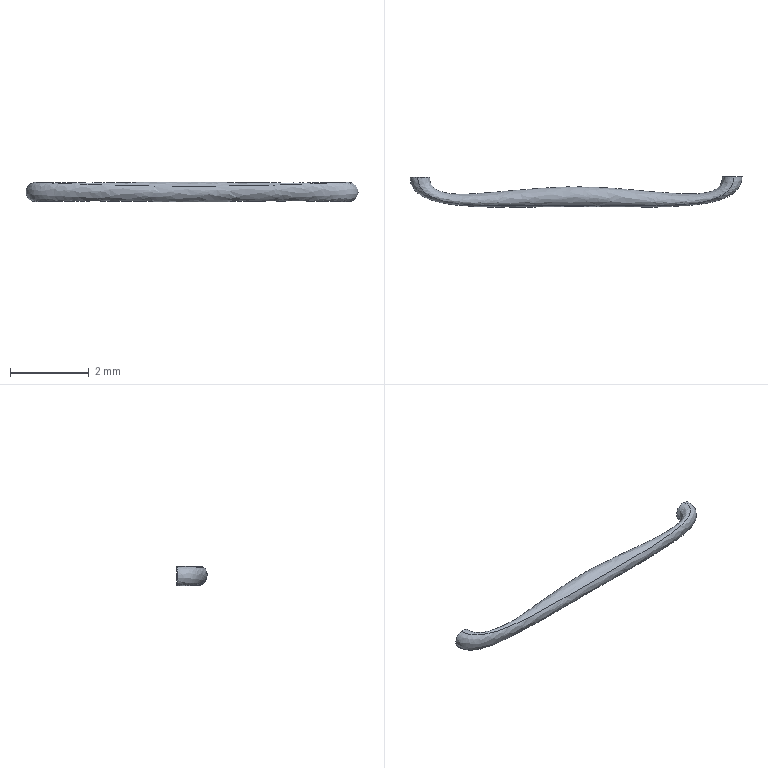Part | SolidWorks | features BaseBody 1 | 1 solid | 4 faces | box 8.423 x 0.7721 x 0.5 mm | volume 1.254 mm3 | plane 2 | spline 2
STEP:
#1=CARTESIAN_POINT('',(345.954,392.468,98.256));
#2=VERTEX_POINT('',#1);
#3=CARTESIAN_POINT('',(345.875,392.468,97.762));
#4=VERTEX_POINT('',#3);
#5=CARTESIAN_POINT('',(345.954,392.468,98.256));
#6=CARTESIAN_POINT('',(345.961,392.468,98.255));
#7=CARTESIAN_POINT('',(345.975,392.468,98.252));
#8=CARTESIAN_POINT('',(345.994,392.468,98.246));
#9=CARTESIAN_POINT('',(346.013,392.468,98.239));
#10=CARTESIAN_POINT('',(346.072,392.468,98.211));
#11=CARTESIAN_POINT('',(346.132,392.468,98.149));
#12=CARTESIAN_POINT('',(346.165,392.468,98.05));
#13=CARTESIAN_POINT('',(346.166,392.468,97.961));
#14=CARTESIAN_POINT('',(346.132,392.468,97.872));
#15=CARTESIAN_POINT('',(346.064,392.468,97.801));
#16=CARTESIAN_POINT('',(345.976,392.468,97.76));
#17=CARTESIAN_POINT('',(345.908,392.468,97.757));
#18=CARTESIAN_POINT('',(345.875,392.468,97.762));
#19=B_SPLINE_CURVE_WITH_KNOTS('',3,(#5,#6,#7,#8,#9,#10,#11,#12,#13,#14,#15,#16,#17,#18),.UNSPECIFIED.,.F.,.F.,(4,1,1,1,1,1,1,1,1,1,1,4),(0.,0.025,0.05,0.075,0.1,0.3,0.4,0.5,0.625,0.75,0.875,1.),.UNSPECIFIED.);
#20=EDGE_CURVE('',#2,#4,#19,.T.);
#21=ORIENTED_EDGE('',*,*,#20,.T.);
#22=CARTESIAN_POINT('',(345.875,392.468,97.762));
#23=CARTESIAN_POINT('',(345.842,392.468,97.767));
#24=CARTESIAN_POINT('',(345.778,392.468,97.792));
#25=CARTESIAN_POINT('',(345.707,392.468,97.859));
#26=CARTESIAN_POINT('',(345.666,392.468,97.947));
#27=CARTESIAN_POINT('',(345.661,392.468,98.043));
#28=CARTESIAN_POINT('',(345.69,392.468,98.127));
#29=CARTESIAN_POINT('',(345.752,392.468,98.21));
#30=CARTESIAN_POINT('',(345.829,392.468,98.25));
#31=CARTESIAN_POINT('',(345.894,392.468,98.258));
#32=CARTESIAN_POINT('',(345.914,392.468,98.259));
#33=CARTESIAN_POINT('',(345.934,392.468,98.258));
#34=CARTESIAN_POINT('',(345.948,392.468,98.257));
#35=CARTESIAN_POINT('',(345.954,392.468,98.256));
#36=B_SPLINE_CURVE_WITH_KNOTS('',3,(#22,#23,#24,#25,#26,#27,#28,#29,#30,#31,#32,#33,#34,#35),.UNSPECIFIED.,.F.,.F.,(4,1,1,1,1,1,1,1,1,1,1,4),(0.,0.125,0.25,0.375,0.5,0.6,0.7,0.9,0.925,0.95,0.975,1.),.UNSPECIFIED.);
#37=EDGE_CURVE('',#4,#2,#36,.T.);
#38=ORIENTED_EDGE('',*,*,#37,.T.);
#39=EDGE_LOOP('',(#21,#38));
#40=FACE_OUTER_BOUND('',#39,.T.);
#41=CARTESIAN_POINT('',(345.915,392.468,98.009));
#42=DIRECTION('',(0.0009599,-1.,0.));
#43=DIRECTION('',(0.,0.,-1.));
#44=AXIS2_PLACEMENT_3D('',#41,#42,#43);
#45=PLANE('',#44);
#46=ADVANCED_FACE('',(#40),#45,.F.);
#47=CARTESIAN_POINT('',(337.94,392.46,98.253));
#48=VERTEX_POINT('',#47);
#49=CARTESIAN_POINT('',(338.044,392.46,97.764));
#50=VERTEX_POINT('',#49);
#51=CARTESIAN_POINT('',(337.94,392.46,98.253));
#52=CARTESIAN_POINT('',(337.946,392.46,98.255));
#53=CARTESIAN_POINT('',(337.96,392.46,98.257));
#54=CARTESIAN_POINT('',(337.98,392.46,98.259));
#55=CARTESIAN_POINT('',(338.,392.46,98.259));
#56=CARTESIAN_POINT('',(338.065,392.46,98.254));
#57=CARTESIAN_POINT('',(338.144,392.46,98.218));
#58=CARTESIAN_POINT('',(338.211,392.46,98.138));
#59=CARTESIAN_POINT('',(338.243,392.46,98.056));
#60=CARTESIAN_POINT('',(338.244,392.46,97.96));
#61=CARTESIAN_POINT('',(338.207,392.46,97.87));
#62=CARTESIAN_POINT('',(338.14,392.46,97.799));
#63=CARTESIAN_POINT('',(338.077,392.46,97.771));
#64=CARTESIAN_POINT('',(338.044,392.46,97.764));
#65=B_SPLINE_CURVE_WITH_KNOTS('',3,(#51,#52,#53,#54,#55,#56,#57,#58,#59,#60,#61,#62,#63,#64),.UNSPECIFIED.,.F.,.F.,(4,1,1,1,1,1,1,1,1,1,1,4),(0.,0.025,0.05,0.075,0.1,0.3,0.4,0.5,0.625,0.75,0.875,1.),.UNSPECIFIED.);
#66=EDGE_CURVE('',#48,#50,#65,.T.);
#67=ORIENTED_EDGE('',*,*,#66,.T.);
#68=CARTESIAN_POINT('',(338.044,392.46,97.764));
#69=CARTESIAN_POINT('',(338.011,392.46,97.757));
#70=CARTESIAN_POINT('',(337.943,392.46,97.757));
#71=CARTESIAN_POINT('',(337.853,392.46,97.794));
#72=CARTESIAN_POINT('',(337.782,392.46,97.861));
#73=CARTESIAN_POINT('',(337.743,392.46,97.949));
#74=CARTESIAN_POINT('',(337.739,392.46,98.038));
#75=CARTESIAN_POINT('',(337.767,392.46,98.138));
#76=CARTESIAN_POINT('',(337.824,392.46,98.203));
#77=CARTESIAN_POINT('',(337.882,392.46,98.234));
#78=CARTESIAN_POINT('',(337.901,392.46,98.242));
#79=CARTESIAN_POINT('',(337.92,392.46,98.248));
#80=CARTESIAN_POINT('',(337.933,392.46,98.252));
#81=CARTESIAN_POINT('',(337.94,392.46,98.253));
#82=B_SPLINE_CURVE_WITH_KNOTS('',3,(#68,#69,#70,#71,#72,#73,#74,#75,#76,#77,#78,#79,#80,#81),.UNSPECIFIED.,.F.,.F.,(4,1,1,1,1,1,1,1,1,1,1,4),(0.,0.125,0.25,0.375,0.5,0.6,0.7,0.9,0.925,0.95,0.975,1.),.UNSPECIFIED.);
#83=EDGE_CURVE('',#50,#48,#82,.T.);
#84=ORIENTED_EDGE('',*,*,#83,.T.);
#85=EDGE_LOOP('',(#67,#84));
#86=FACE_OUTER_BOUND('',#85,.T.);
#87=CARTESIAN_POINT('',(337.992,392.46,98.009));
#88=DIRECTION('',(0.0009599,-1.,0.));
#89=DIRECTION('',(0.,0.,-1.));
#90=AXIS2_PLACEMENT_3D('',#87,#88,#89);
#91=PLANE('',#90);
#92=ADVANCED_FACE('',(#86),#91,.F.);
#93=CARTESIAN_POINT('',(338.044,392.46,97.764));
#94=CARTESIAN_POINT('',(338.045,391.637,97.764));
#95=CARTESIAN_POINT('',(341.947,392.702,97.981));
#96=CARTESIAN_POINT('',(345.876,391.642,97.762));
#97=CARTESIAN_POINT('',(345.875,392.468,97.762));
#98=B_SPLINE_CURVE_WITH_KNOTS('',3,(#93,#94,#95,#96,#97),.UNSPECIFIED.,.F.,.F.,(4,1,4),(0.,0.5,1.),.UNSPECIFIED.);
#99=EDGE_CURVE('',#50,#4,#98,.T.);
#100=ORIENTED_EDGE('',*,*,#99,.T.);
#101=ORIENTED_EDGE('',*,*,#20,.F.);
#102=CARTESIAN_POINT('',(345.954,392.468,98.256));
#103=CARTESIAN_POINT('',(345.955,391.561,98.256));
#104=CARTESIAN_POINT('',(341.96,391.959,98.052));
#105=CARTESIAN_POINT('',(337.94,391.551,98.253));
#106=CARTESIAN_POINT('',(337.94,392.46,98.253));
#107=B_SPLINE_CURVE_WITH_KNOTS('',3,(#102,#103,#104,#105,#106),.UNSPECIFIED.,.F.,.F.,(4,1,4),(0.,0.5,1.),.UNSPECIFIED.);
#108=EDGE_CURVE('',#2,#48,#107,.T.);
#109=ORIENTED_EDGE('',*,*,#108,.T.);
#110=ORIENTED_EDGE('',*,*,#83,.F.);
#111=EDGE_LOOP('',(#100,#101,#109,#110));
#112=FACE_OUTER_BOUND('',#111,.T.);
#113=CARTESIAN_POINT('',(337.961,392.546,98.256));
#114=CARTESIAN_POINT('',(337.834,391.542,98.262));
#115=CARTESIAN_POINT('',(341.966,391.986,98.069));
#116=CARTESIAN_POINT('',(346.071,391.552,98.264));
#117=CARTESIAN_POINT('',(345.932,392.561,98.257));
#118=CARTESIAN_POINT('',(337.955,392.546,98.255));
#119=CARTESIAN_POINT('',(337.828,391.541,98.261));
#120=CARTESIAN_POINT('',(341.966,391.981,98.061));
#121=CARTESIAN_POINT('',(346.077,391.55,98.264));
#122=CARTESIAN_POINT('',(345.937,392.561,98.257));
#123=CARTESIAN_POINT('',(337.944,392.547,98.253));
#124=CARTESIAN_POINT('',(337.816,391.538,98.259));
#125=CARTESIAN_POINT('',(341.966,391.97,98.043));
#126=CARTESIAN_POINT('',(346.089,391.547,98.263));
#127=CARTESIAN_POINT('',(345.949,392.562,98.255));
#128=CARTESIAN_POINT('',(337.925,392.547,98.248));
#129=CARTESIAN_POINT('',(337.797,391.532,98.255));
#130=CARTESIAN_POINT('',(341.965,391.955,98.014));
#131=CARTESIAN_POINT('',(346.108,391.542,98.26));
#132=CARTESIAN_POINT('',(345.968,392.562,98.251));
#133=CARTESIAN_POINT('',(337.906,392.548,98.242));
#134=CARTESIAN_POINT('',(337.777,391.527,98.25));
#135=CARTESIAN_POINT('',(341.965,391.942,97.984));
#136=CARTESIAN_POINT('',(346.128,391.537,98.255));
#137=CARTESIAN_POINT('',(345.987,392.563,98.246));
#138=CARTESIAN_POINT('',(337.888,392.548,98.233));
#139=CARTESIAN_POINT('',(337.759,391.522,98.242));
#140=CARTESIAN_POINT('',(341.965,391.932,97.954));
#141=CARTESIAN_POINT('',(346.148,391.532,98.248));
#142=CARTESIAN_POINT('',(346.006,392.563,98.239));
#143=CARTESIAN_POINT('',(337.83,392.55,98.202));
#144=CARTESIAN_POINT('',(337.699,391.508,98.213));
#145=CARTESIAN_POINT('',(341.964,391.906,97.856));
#146=CARTESIAN_POINT('',(346.209,391.517,98.223));
#147=CARTESIAN_POINT('',(346.065,392.565,98.21));
#148=CARTESIAN_POINT('',(337.773,392.55,98.137));
#149=CARTESIAN_POINT('',(337.64,391.497,98.149));
#150=CARTESIAN_POINT('',(341.963,391.924,97.745));
#151=CARTESIAN_POINT('',(346.271,391.505,98.162));
#152=CARTESIAN_POINT('',(346.125,392.566,98.148));
#153=CARTESIAN_POINT('',(337.745,392.55,98.037));
#154=CARTESIAN_POINT('',(337.611,391.497,98.049));
#155=CARTESIAN_POINT('',(341.96,392.023,97.662));
#156=CARTESIAN_POINT('',(346.306,391.504,98.063));
#157=CARTESIAN_POINT('',(346.158,392.566,98.05));
#158=CARTESIAN_POINT('',(337.749,392.549,97.948));
#159=CARTESIAN_POINT('',(337.616,391.504,97.958));
#160=CARTESIAN_POINT('',(341.958,392.145,97.629));
#161=CARTESIAN_POINT('',(346.306,391.51,97.972));
#162=CARTESIAN_POINT('',(346.159,392.565,97.961));
#163=CARTESIAN_POINT('',(337.788,392.548,97.861));
#164=CARTESIAN_POINT('',(337.656,391.522,97.867));
#165=CARTESIAN_POINT('',(341.955,392.305,97.648));
#166=CARTESIAN_POINT('',(346.271,391.527,97.879));
#167=CARTESIAN_POINT('',(346.125,392.563,97.872));
#168=CARTESIAN_POINT('',(337.858,392.545,97.794));
#169=CARTESIAN_POINT('',(337.729,391.548,97.796));
#170=CARTESIAN_POINT('',(341.953,392.474,97.722));
#171=CARTESIAN_POINT('',(346.201,391.552,97.804));
#172=CARTESIAN_POINT('',(346.058,392.56,97.801));
#173=CARTESIAN_POINT('',(337.948,392.542,97.757));
#174=CARTESIAN_POINT('',(337.821,391.578,97.755));
#175=CARTESIAN_POINT('',(341.952,392.626,97.837));
#176=CARTESIAN_POINT('',(346.111,391.58,97.757));
#177=CARTESIAN_POINT('',(345.97,392.557,97.76));
#178=CARTESIAN_POINT('',(338.022,392.54,97.758));
#179=CARTESIAN_POINT('',(337.897,391.597,97.752));
#180=CARTESIAN_POINT('',(341.951,392.713,97.945));
#181=CARTESIAN_POINT('',(346.034,391.6,97.75));
#182=CARTESIAN_POINT('',(345.896,392.555,97.757));
#183=CARTESIAN_POINT('',(338.06,392.539,97.767));
#184=CARTESIAN_POINT('',(337.936,391.606,97.76));
#185=CARTESIAN_POINT('',(341.951,392.745,98.003));
#186=CARTESIAN_POINT('',(345.995,391.609,97.756));
#187=CARTESIAN_POINT('',(345.858,392.554,97.764));
#188=CARTESIAN_POINT('',(338.064,392.539,97.768));
#189=CARTESIAN_POINT('',(337.941,391.607,97.761));
#190=CARTESIAN_POINT('',(341.951,392.749,98.011));
#191=CARTESIAN_POINT('',(345.99,391.61,97.757));
#192=CARTESIAN_POINT('',(345.853,392.554,97.765));
#193=B_SPLINE_SURFACE_WITH_KNOTS('',3,3,((#113,#114,#115,#116,#117),(#118,#119,#120,#121,#122),(#123,#124,#125,#126,#127),(#128,#129,#130,#131,#132),(#133,#134,#135,#136,#137),(#138,#139,#140,#141,#142),(#143,#144,#145,#146,#147),(#148,#149,#150,#151,#152),(#153,#154,#155,#156,#157),(#158,#159,#160,#161,#162),(#163,#164,#165,#166,#167),(#168,#169,#170,#171,#172),(#173,#174,#175,#176,#177),(#178,#179,#180,#181,#182),(#183,#184,#185,#186,#187),(#188,#189,#190,#191,#192)),.UNSPECIFIED.,.F.,.F.,.F.,(4,1,1,1,1,1,1,1,1,1,1,1,1,4),(4,1,4),(-0.009538,0.,0.0125,0.025,0.0375,0.05,0.15,0.2,0.25,0.3125,0.375,0.4375,0.5,0.5095),(-0.01527,0.5,1.017),.UNSPECIFIED.);
#194=ADVANCED_FACE('',(#112),#193,.T.);
#195=ORIENTED_EDGE('',*,*,#66,.F.);
#196=ORIENTED_EDGE('',*,*,#108,.F.);
#197=ORIENTED_EDGE('',*,*,#37,.F.);
#198=ORIENTED_EDGE('',*,*,#99,.F.);
#199=EDGE_LOOP('',(#195,#196,#197,#198));
#200=FACE_OUTER_BOUND('',#199,.T.);
#201=CARTESIAN_POINT('',(338.034,392.54,97.762));
#202=CARTESIAN_POINT('',(337.91,391.6,97.756));
#203=CARTESIAN_POINT('',(341.951,392.722,97.965));
#204=CARTESIAN_POINT('',(346.021,391.603,97.753));
#205=CARTESIAN_POINT('',(345.883,392.555,97.76));
#206=CARTESIAN_POINT('',(338.04,392.54,97.763));
#207=CARTESIAN_POINT('',(337.915,391.601,97.756));
#208=CARTESIAN_POINT('',(341.951,392.727,97.972));
#209=CARTESIAN_POINT('',(346.016,391.604,97.754));
#210=CARTESIAN_POINT('',(345.878,392.555,97.761));
#211=CARTESIAN_POINT('',(338.078,392.539,97.77));
#212=CARTESIAN_POINT('',(337.955,391.611,97.761));
#213=CARTESIAN_POINT('',(341.951,392.763,98.031));
#214=CARTESIAN_POINT('',(345.976,391.613,97.757));
#215=CARTESIAN_POINT('',(345.84,392.553,97.766));
#216=CARTESIAN_POINT('',(338.145,392.538,97.8));
#217=CARTESIAN_POINT('',(338.024,391.626,97.789));
#218=CARTESIAN_POINT('',(341.952,392.804,98.141));
#219=CARTESIAN_POINT('',(345.905,391.628,97.78));
#220=CARTESIAN_POINT('',(345.771,392.552,97.792));
#221=CARTESIAN_POINT('',(338.212,392.536,97.87));
#222=CARTESIAN_POINT('',(338.093,391.64,97.858));
#223=CARTESIAN_POINT('',(341.954,392.789,98.269));
#224=CARTESIAN_POINT('',(345.832,391.643,97.846));
#225=CARTESIAN_POINT('',(345.701,392.55,97.86));
#226=CARTESIAN_POINT('',(338.249,392.536,97.96));
#227=CARTESIAN_POINT('',(338.131,391.645,97.948));
#228=CARTESIAN_POINT('',(341.956,392.713,98.362));
#229=CARTESIAN_POINT('',(345.789,391.649,97.934));
#230=CARTESIAN_POINT('',(345.659,392.55,97.948));
#231=CARTESIAN_POINT('',(338.248,392.537,98.056));
#232=CARTESIAN_POINT('',(338.131,391.64,98.045));
#233=CARTESIAN_POINT('',(341.959,392.584,98.402));
#234=CARTESIAN_POINT('',(345.785,391.646,98.031));
#235=CARTESIAN_POINT('',(345.655,392.55,98.043));
#236=CARTESIAN_POINT('',(338.216,392.538,98.139));
#237=CARTESIAN_POINT('',(338.097,391.626,98.131));
#238=CARTESIAN_POINT('',(341.961,392.436,98.39));
#239=CARTESIAN_POINT('',(345.814,391.633,98.119));
#240=CARTESIAN_POINT('',(345.683,392.552,98.128));
#241=CARTESIAN_POINT('',(338.15,392.541,98.218));
#242=CARTESIAN_POINT('',(338.029,391.602,98.215));
#243=CARTESIAN_POINT('',(341.964,392.253,98.328));
#244=CARTESIAN_POINT('',(345.878,391.61,98.206));
#245=CARTESIAN_POINT('',(345.745,392.555,98.21));
#246=CARTESIAN_POINT('',(338.071,392.543,98.254));
#247=CARTESIAN_POINT('',(337.947,391.575,98.255));
#248=CARTESIAN_POINT('',(341.965,392.116,98.229));
#249=CARTESIAN_POINT('',(345.957,391.584,98.251));
#250=CARTESIAN_POINT('',(345.822,392.557,98.25));
#251=CARTESIAN_POINT('',(338.005,392.545,98.259));
#252=CARTESIAN_POINT('',(337.88,391.555,98.263));
#253=CARTESIAN_POINT('',(341.965,392.034,98.135));
#254=CARTESIAN_POINT('',(346.025,391.565,98.262));
#255=CARTESIAN_POINT('',(345.887,392.56,98.258));
#256=CARTESIAN_POINT('',(337.986,392.546,98.259));
#257=CARTESIAN_POINT('',(337.859,391.55,98.263));
#258=CARTESIAN_POINT('',(341.966,392.011,98.106));
#259=CARTESIAN_POINT('',(346.045,391.559,98.264));
#260=CARTESIAN_POINT('',(345.907,392.56,98.259));
#261=CARTESIAN_POINT('',(337.965,392.546,98.257));
#262=CARTESIAN_POINT('',(337.839,391.544,98.262));
#263=CARTESIAN_POINT('',(341.966,391.99,98.076));
#264=CARTESIAN_POINT('',(346.066,391.553,98.264));
#265=CARTESIAN_POINT('',(345.927,392.561,98.258));
#266=CARTESIAN_POINT('',(337.947,392.547,98.254));
#267=CARTESIAN_POINT('',(337.819,391.538,98.26));
#268=CARTESIAN_POINT('',(341.966,391.973,98.048));
#269=CARTESIAN_POINT('',(346.086,391.548,98.263));
#270=CARTESIAN_POINT('',(345.946,392.561,98.256));
#271=CARTESIAN_POINT('',(337.935,392.547,98.251));
#272=CARTESIAN_POINT('',(337.807,391.535,98.258));
#273=CARTESIAN_POINT('',(341.965,391.963,98.029));
#274=CARTESIAN_POINT('',(346.098,391.545,98.261));
#275=CARTESIAN_POINT('',(345.958,392.562,98.253));
#276=CARTESIAN_POINT('',(337.93,392.547,98.249));
#277=CARTESIAN_POINT('',(337.802,391.534,98.256));
#278=CARTESIAN_POINT('',(341.965,391.959,98.022));
#279=CARTESIAN_POINT('',(346.103,391.543,98.26));
#280=CARTESIAN_POINT('',(345.963,392.562,98.252));
#281=B_SPLINE_SURFACE_WITH_KNOTS('',3,3,((#201,#202,#203,#204,#205),(#206,#207,#208,#209,#210),(#211,#212,#213,#214,#215),(#216,#217,#218,#219,#220),(#221,#222,#223,#224,#225),(#226,#227,#228,#229,#230),(#231,#232,#233,#234,#235),(#236,#237,#238,#239,#240),(#241,#242,#243,#244,#245),(#246,#247,#248,#249,#250),(#251,#252,#253,#254,#255),(#256,#257,#258,#259,#260),(#261,#262,#263,#264,#265),(#266,#267,#268,#269,#270),(#271,#272,#273,#274,#275),(#276,#277,#278,#279,#280)),.UNSPECIFIED.,.F.,.F.,.F.,(4,1,1,1,1,1,1,1,1,1,1,1,1,4),(4,1,4),(0.4905,0.5,0.5625,0.625,0.6875,0.75,0.8,0.85,0.95,0.9625,0.975,0.9875,1.,1.01),(-0.01527,0.5,1.017),.UNSPECIFIED.);
#282=ADVANCED_FACE('',(#200),#281,.T.);
#283=CLOSED_SHELL('',(#46,#92,#194,#282));
#284=MANIFOLD_SOLID_BREP('',#283);
#285=CARTESIAN_POINT('',(0.,0.,0.));
#286=DIRECTION('',(0.,0.,1.));
#287=DIRECTION('',(1.,0.,0.));
#288=AXIS2_PLACEMENT_3D('',#285,#286,#287);
#289=(LENGTH_UNIT()NAMED_UNIT(*)SI_UNIT(.MILLI.,.METRE.));
#290=UNCERTAINTY_MEASURE_WITH_UNIT(LENGTH_MEASURE(0.00001),#289,'','');
#291=(NAMED_UNIT(*)PLANE_ANGLE_UNIT()SI_UNIT($,.RADIAN.));
#292=(NAMED_UNIT(*)SI_UNIT($,.STERADIAN.)SOLID_ANGLE_UNIT());
#293=(GEOMETRIC_REPRESENTATION_CONTEXT(3)GLOBAL_UNCERTAINTY_ASSIGNED_CONTEXT((#290))GLOBAL_UNIT_ASSIGNED_CONTEXT((#289,#291,#292))REPRESENTATION_CONTEXT('',''));
#294=ADVANCED_BREP_SHAPE_REPRESENTATION('',(#284,#288),#293);